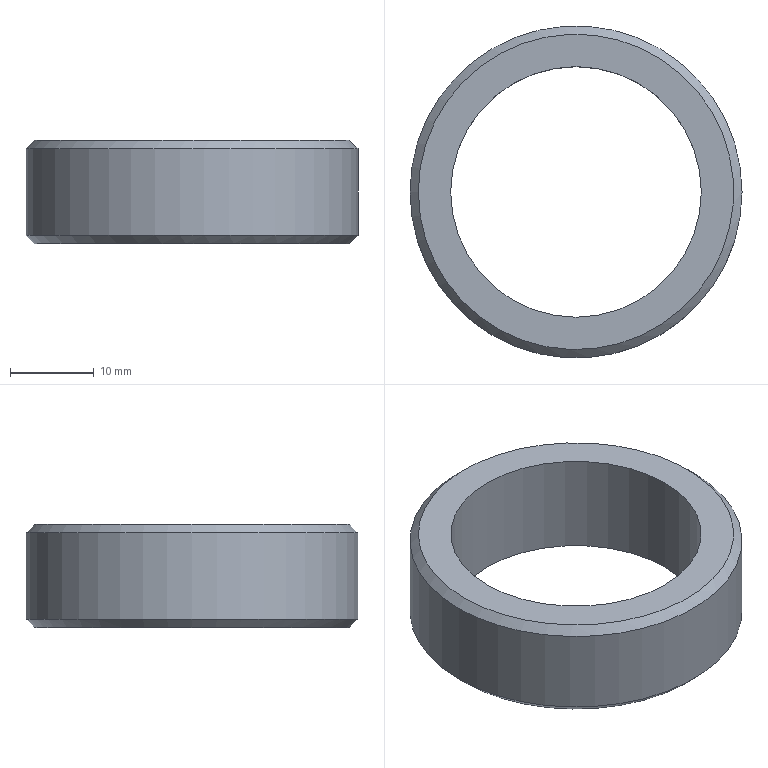Part | NX | features CHAMFER 2, DATUM_CSYS 2, EXTRUDE 1, SKETCH 1 | 1 solid | 6 faces | box 39.74 x 39.74 x 12.34 mm | volume 6461 mm3 | cylinder 2 | plane 2 | cone 2 | commonest cylinder face diameters 30 x1 39.74 x1
STEP:
#1=CARTESIAN_POINT('',(-19.87,0.,1.));
#2=VERTEX_POINT('',#1);
#3=CARTESIAN_POINT('',(0.,0.,1.));
#4=DIRECTION('',(0.,0.,-1.));
#5=DIRECTION('',(-1.,0.,0.));
#6=AXIS2_PLACEMENT_3D('',#3,#4,#5);
#7=CIRCLE('',#6,19.87);
#8=EDGE_CURVE('',#2,#2,#7,.F.);
#9=ORIENTED_EDGE('',*,*,#8,.T.);
#10=EDGE_LOOP('',(#9));
#11=FACE_BOUND('',#10,.T.);
#12=CARTESIAN_POINT('',(-19.87,0.,11.34));
#13=VERTEX_POINT('',#12);
#14=CARTESIAN_POINT('',(0.,0.,11.34));
#15=DIRECTION('',(0.,0.,-1.));
#16=DIRECTION('',(-1.,0.,0.));
#17=AXIS2_PLACEMENT_3D('',#14,#15,#16);
#18=CIRCLE('',#17,19.87);
#19=EDGE_CURVE('',#13,#13,#18,.T.);
#20=ORIENTED_EDGE('',*,*,#19,.T.);
#21=EDGE_LOOP('',(#20));
#22=FACE_BOUND('',#21,.T.);
#23=CARTESIAN_POINT('',(0.,0.,12.34));
#24=DIRECTION('',(0.,0.,-1.));
#25=DIRECTION('',(-1.,0.,0.));
#26=AXIS2_PLACEMENT_3D('',#23,#24,#25);
#27=CYLINDRICAL_SURFACE('',#26,19.87);
#28=ADVANCED_FACE('',(#11,#22),#27,.T.);
#29=CARTESIAN_POINT('',(15.,0.,12.34));
#30=VERTEX_POINT('',#29);
#31=CARTESIAN_POINT('',(0.,0.,12.34));
#32=DIRECTION('',(0.,0.,-1.));
#33=DIRECTION('',(1.,0.,0.));
#34=AXIS2_PLACEMENT_3D('',#31,#32,#33);
#35=CIRCLE('',#34,15.);
#36=EDGE_CURVE('',#30,#30,#35,.T.);
#37=ORIENTED_EDGE('',*,*,#36,.F.);
#38=EDGE_LOOP('',(#37));
#39=FACE_BOUND('',#38,.T.);
#40=CARTESIAN_POINT('',(15.,0.,0.));
#41=VERTEX_POINT('',#40);
#42=CARTESIAN_POINT('',(0.,0.,0.));
#43=DIRECTION('',(0.,0.,-1.));
#44=DIRECTION('',(1.,0.,0.));
#45=AXIS2_PLACEMENT_3D('',#42,#43,#44);
#46=CIRCLE('',#45,15.);
#47=EDGE_CURVE('',#41,#41,#46,.T.);
#48=ORIENTED_EDGE('',*,*,#47,.T.);
#49=EDGE_LOOP('',(#48));
#50=FACE_BOUND('',#49,.T.);
#51=CARTESIAN_POINT('',(0.,0.,12.34));
#52=DIRECTION('',(0.,0.,-1.));
#53=DIRECTION('',(-1.,0.,0.));
#54=AXIS2_PLACEMENT_3D('',#51,#52,#53);
#55=CYLINDRICAL_SURFACE('',#54,15.);
#56=ADVANCED_FACE('',(#39,#50),#55,.F.);
#57=CARTESIAN_POINT('',(-18.87,0.,12.34));
#58=VERTEX_POINT('',#57);
#59=CARTESIAN_POINT('',(0.,0.,12.34));
#60=DIRECTION('',(0.,0.,-1.));
#61=DIRECTION('',(-1.,0.,0.));
#62=AXIS2_PLACEMENT_3D('',#59,#60,#61);
#63=CIRCLE('',#62,18.87);
#64=EDGE_CURVE('',#58,#58,#63,.F.);
#65=ORIENTED_EDGE('',*,*,#64,.T.);
#66=EDGE_LOOP('',(#65));
#67=FACE_BOUND('',#66,.T.);
#68=ORIENTED_EDGE('',*,*,#36,.T.);
#69=EDGE_LOOP('',(#68));
#70=FACE_BOUND('',#69,.T.);
#71=CARTESIAN_POINT('',(0.,0.,12.34));
#72=DIRECTION('',(0.,0.,-1.));
#73=DIRECTION('',(-1.,0.,0.));
#74=AXIS2_PLACEMENT_3D('',#71,#72,#73);
#75=PLANE('',#74);
#76=ADVANCED_FACE('',(#67,#70),#75,.F.);
#77=CARTESIAN_POINT('',(-18.87,0.,0.));
#78=VERTEX_POINT('',#77);
#79=CARTESIAN_POINT('',(0.,0.,0.));
#80=DIRECTION('',(0.,0.,-1.));
#81=DIRECTION('',(-1.,0.,0.));
#82=AXIS2_PLACEMENT_3D('',#79,#80,#81);
#83=CIRCLE('',#82,18.87);
#84=EDGE_CURVE('',#78,#78,#83,.T.);
#85=ORIENTED_EDGE('',*,*,#84,.T.);
#86=EDGE_LOOP('',(#85));
#87=FACE_BOUND('',#86,.T.);
#88=ORIENTED_EDGE('',*,*,#47,.F.);
#89=EDGE_LOOP('',(#88));
#90=FACE_BOUND('',#89,.T.);
#91=CARTESIAN_POINT('',(0.,0.,0.));
#92=DIRECTION('',(0.,0.,-1.));
#93=DIRECTION('',(-1.,0.,0.));
#94=AXIS2_PLACEMENT_3D('',#91,#92,#93);
#95=PLANE('',#94);
#96=ADVANCED_FACE('',(#87,#90),#95,.T.);
#97=ORIENTED_EDGE('',*,*,#64,.F.);
#98=EDGE_LOOP('',(#97));
#99=FACE_BOUND('',#98,.T.);
#100=ORIENTED_EDGE('',*,*,#19,.F.);
#101=EDGE_LOOP('',(#100));
#102=FACE_BOUND('',#101,.T.);
#103=CARTESIAN_POINT('',(0.,0.,11.34));
#104=DIRECTION('',(0.,0.,-1.));
#105=DIRECTION('',(-1.,0.,0.));
#106=AXIS2_PLACEMENT_3D('',#103,#104,#105);
#107=CONICAL_SURFACE('',#106,19.87,0.7854);
#108=ADVANCED_FACE('',(#99,#102),#107,.T.);
#109=ORIENTED_EDGE('',*,*,#8,.F.);
#110=EDGE_LOOP('',(#109));
#111=FACE_BOUND('',#110,.T.);
#112=ORIENTED_EDGE('',*,*,#84,.F.);
#113=EDGE_LOOP('',(#112));
#114=FACE_BOUND('',#113,.T.);
#115=CARTESIAN_POINT('',(0.,0.,0.));
#116=DIRECTION('',(0.,0.,1.));
#117=DIRECTION('',(1.,0.,0.));
#118=AXIS2_PLACEMENT_3D('',#115,#116,#117);
#119=CONICAL_SURFACE('',#118,18.87,0.7854);
#120=ADVANCED_FACE('',(#111,#114),#119,.T.);
#121=CLOSED_SHELL('',(#28,#56,#76,#96,#108,#120));
#122=MANIFOLD_SOLID_BREP('',#121);
#123=(LENGTH_UNIT()NAMED_UNIT(*)SI_UNIT(.MILLI.,.METRE.));
#124=UNCERTAINTY_MEASURE_WITH_UNIT(LENGTH_MEASURE(0.00001),#123,'','');
#125=(NAMED_UNIT(*)PLANE_ANGLE_UNIT()SI_UNIT($,.RADIAN.));
#126=(NAMED_UNIT(*)SI_UNIT($,.STERADIAN.)SOLID_ANGLE_UNIT());
#127=(GEOMETRIC_REPRESENTATION_CONTEXT(3)GLOBAL_UNCERTAINTY_ASSIGNED_CONTEXT((#124))GLOBAL_UNIT_ASSIGNED_CONTEXT((#123,#125,#126))REPRESENTATION_CONTEXT('',''));
#128=ADVANCED_BREP_SHAPE_REPRESENTATION('',(#122),#127);